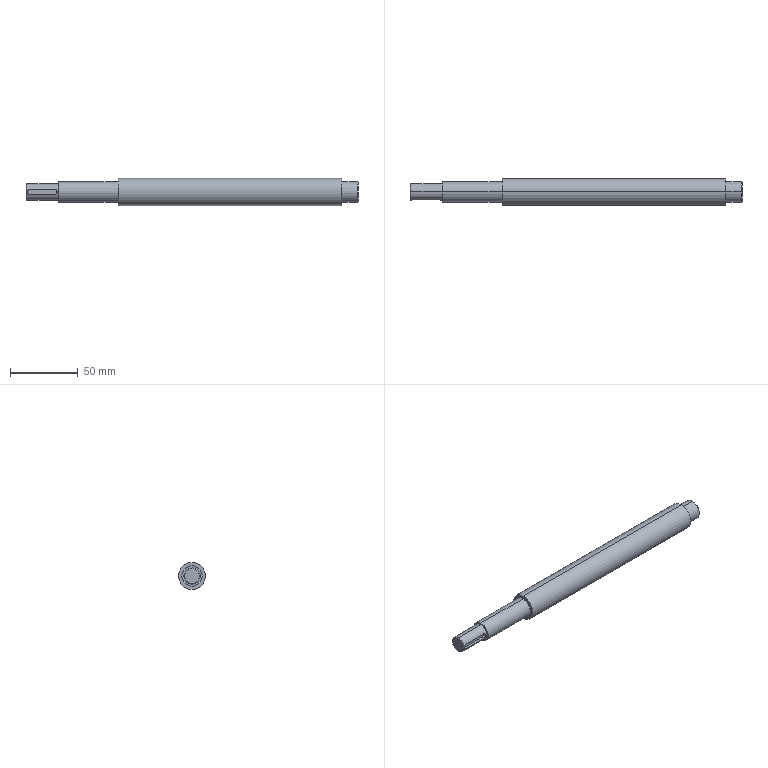Part | SolidWorks | features Chamfer 1, ICE 1, Revolution 1 | 1 solid | 22 faces | box 245 x 20 x 20 mm | volume 64259 mm3 | cylinder 10 | plane 8 | cone 4 | commonest cylinder face diameters 15 x4 4 x2 12 x2 20 x2
STEP:
#1=CARTESIAN_POINT('',(0.,0.,5.5));
#2=VERTEX_POINT('',#1);
#3=CARTESIAN_POINT('',(0.,0.,-5.5));
#4=VERTEX_POINT('',#3);
#5=CARTESIAN_POINT('',(0.,0.,0.));
#6=DIRECTION('',(-1.,0.,0.));
#7=DIRECTION('',(0.,0.,-1.));
#8=AXIS2_PLACEMENT_3D('',#5,#6,#7);
#9=CIRCLE('',#8,5.5);
#10=EDGE_CURVE('',#2,#4,#9,.T.);
#11=ORIENTED_EDGE('',*,*,#10,.F.);
#12=CARTESIAN_POINT('',(0.5,0.,6.));
#13=VERTEX_POINT('',#12);
#14=CARTESIAN_POINT('',(0.,0.,5.5));
#15=DIRECTION('',(0.7071,0.,0.7071));
#16=VECTOR('',#15,1000.);
#17=LINE('',#14,#16);
#18=EDGE_CURVE('',#2,#13,#17,.T.);
#19=ORIENTED_EDGE('',*,*,#18,.T.);
#20=CARTESIAN_POINT('',(0.5,0.,-6.));
#21=VERTEX_POINT('',#20);
#22=CARTESIAN_POINT('',(0.5,0.,0.));
#23=DIRECTION('',(1.,0.,0.));
#24=DIRECTION('',(0.,0.,-1.));
#25=AXIS2_PLACEMENT_3D('',#22,#23,#24);
#26=CIRCLE('',#25,6.);
#27=EDGE_CURVE('',#21,#13,#26,.T.);
#28=ORIENTED_EDGE('',*,*,#27,.F.);
#29=CARTESIAN_POINT('',(0.,0.,-5.5));
#30=DIRECTION('',(0.7071,0.,-0.7071));
#31=VECTOR('',#30,1000.);
#32=LINE('',#29,#31);
#33=EDGE_CURVE('',#4,#21,#32,.T.);
#34=ORIENTED_EDGE('',*,*,#33,.F.);
#35=EDGE_LOOP('',(#11,#19,#28,#34));
#36=FACE_OUTER_BOUND('',#35,.T.);
#37=CARTESIAN_POINT('',(0.,0.,0.));
#38=DIRECTION('',(1.,0.,0.));
#39=DIRECTION('',(0.,0.,-1.));
#40=AXIS2_PLACEMENT_3D('',#37,#38,#39);
#41=CONICAL_SURFACE('',#40,5.5,0.7854);
#42=ADVANCED_FACE('',(#36),#41,.T.);
#43=CARTESIAN_POINT('',(245.,0.,-7.));
#44=VERTEX_POINT('',#43);
#45=CARTESIAN_POINT('',(245.,0.,7.));
#46=VERTEX_POINT('',#45);
#47=CARTESIAN_POINT('',(245.,0.,0.));
#48=DIRECTION('',(1.,0.,0.));
#49=DIRECTION('',(0.,0.,1.));
#50=AXIS2_PLACEMENT_3D('',#47,#48,#49);
#51=CIRCLE('',#50,7.);
#52=EDGE_CURVE('',#44,#46,#51,.T.);
#53=ORIENTED_EDGE('',*,*,#52,.F.);
#54=CARTESIAN_POINT('',(244.5,0.,-7.5));
#55=VERTEX_POINT('',#54);
#56=CARTESIAN_POINT('',(244.5,0.,-7.5));
#57=DIRECTION('',(-0.7071,0.,-0.7071));
#58=VECTOR('',#57,1000.);
#59=LINE('',#56,#58);
#60=EDGE_CURVE('',#44,#55,#59,.T.);
#61=ORIENTED_EDGE('',*,*,#60,.T.);
#62=CARTESIAN_POINT('',(244.5,0.,7.5));
#63=VERTEX_POINT('',#62);
#64=CARTESIAN_POINT('',(244.5,0.,0.));
#65=DIRECTION('',(-1.,0.,0.));
#66=DIRECTION('',(0.,0.,1.));
#67=AXIS2_PLACEMENT_3D('',#64,#65,#66);
#68=CIRCLE('',#67,7.5);
#69=EDGE_CURVE('',#63,#55,#68,.T.);
#70=ORIENTED_EDGE('',*,*,#69,.F.);
#71=CARTESIAN_POINT('',(244.5,0.,7.5));
#72=DIRECTION('',(-0.7071,0.,0.7071));
#73=VECTOR('',#72,1000.);
#74=LINE('',#71,#73);
#75=EDGE_CURVE('',#46,#63,#74,.T.);
#76=ORIENTED_EDGE('',*,*,#75,.F.);
#77=EDGE_LOOP('',(#53,#61,#70,#76));
#78=FACE_OUTER_BOUND('',#77,.T.);
#79=CARTESIAN_POINT('',(244.5,0.,0.));
#80=DIRECTION('',(-1.,0.,0.));
#81=DIRECTION('',(0.,0.,1.));
#82=AXIS2_PLACEMENT_3D('',#79,#80,#81);
#83=CONICAL_SURFACE('',#82,7.5,0.7854);
#84=ADVANCED_FACE('',(#78),#83,.T.);
#85=ORIENTED_EDGE('',*,*,#69,.T.);
#86=CARTESIAN_POINT('',(233.,0.,-7.5));
#87=VERTEX_POINT('',#86);
#88=CARTESIAN_POINT('',(0.,0.,-7.5));
#89=DIRECTION('',(-1.,0.,0.));
#90=VECTOR('',#89,1000.);
#91=LINE('',#88,#90);
#92=EDGE_CURVE('',#55,#87,#91,.T.);
#93=ORIENTED_EDGE('',*,*,#92,.T.);
#94=CARTESIAN_POINT('',(233.,0.,7.5));
#95=VERTEX_POINT('',#94);
#96=CARTESIAN_POINT('',(233.,0.,0.));
#97=DIRECTION('',(-1.,0.,0.));
#98=DIRECTION('',(0.,0.,1.));
#99=AXIS2_PLACEMENT_3D('',#96,#97,#98);
#100=CIRCLE('',#99,7.5);
#101=EDGE_CURVE('',#95,#87,#100,.T.);
#102=ORIENTED_EDGE('',*,*,#101,.F.);
#103=CARTESIAN_POINT('',(0.,0.,7.5));
#104=DIRECTION('',(-1.,0.,0.));
#105=VECTOR('',#104,1000.);
#106=LINE('',#103,#105);
#107=EDGE_CURVE('',#63,#95,#106,.T.);
#108=ORIENTED_EDGE('',*,*,#107,.F.);
#109=EDGE_LOOP('',(#85,#93,#102,#108));
#110=FACE_OUTER_BOUND('',#109,.T.);
#111=CARTESIAN_POINT('',(0.,0.,0.));
#112=DIRECTION('',(-1.,0.,0.));
#113=DIRECTION('',(0.,0.,1.));
#114=AXIS2_PLACEMENT_3D('',#111,#112,#113);
#115=CYLINDRICAL_SURFACE('',#114,7.5);
#116=ADVANCED_FACE('',(#110),#115,.T.);
#117=CARTESIAN_POINT('',(233.,0.,10.));
#118=VERTEX_POINT('',#117);
#119=CARTESIAN_POINT('',(233.,0.,-10.));
#120=VERTEX_POINT('',#119);
#121=CARTESIAN_POINT('',(233.,0.,0.));
#122=DIRECTION('',(-1.,0.,0.));
#123=DIRECTION('',(0.,0.,1.));
#124=AXIS2_PLACEMENT_3D('',#121,#122,#123);
#125=CIRCLE('',#124,10.);
#126=EDGE_CURVE('',#118,#120,#125,.T.);
#127=ORIENTED_EDGE('',*,*,#126,.T.);
#128=CARTESIAN_POINT('',(68.,0.,-10.));
#129=VERTEX_POINT('',#128);
#130=CARTESIAN_POINT('',(0.,0.,-10.));
#131=DIRECTION('',(-1.,0.,0.));
#132=VECTOR('',#131,1000.);
#133=LINE('',#130,#132);
#134=EDGE_CURVE('',#120,#129,#133,.T.);
#135=ORIENTED_EDGE('',*,*,#134,.T.);
#136=CARTESIAN_POINT('',(68.,0.,10.));
#137=VERTEX_POINT('',#136);
#138=CARTESIAN_POINT('',(68.,0.,0.));
#139=DIRECTION('',(-1.,0.,0.));
#140=DIRECTION('',(0.,0.,1.));
#141=AXIS2_PLACEMENT_3D('',#138,#139,#140);
#142=CIRCLE('',#141,10.);
#143=EDGE_CURVE('',#137,#129,#142,.T.);
#144=ORIENTED_EDGE('',*,*,#143,.F.);
#145=CARTESIAN_POINT('',(0.,0.,10.));
#146=DIRECTION('',(-1.,0.,0.));
#147=VECTOR('',#146,1000.);
#148=LINE('',#145,#147);
#149=EDGE_CURVE('',#118,#137,#148,.T.);
#150=ORIENTED_EDGE('',*,*,#149,.F.);
#151=EDGE_LOOP('',(#127,#135,#144,#150));
#152=FACE_OUTER_BOUND('',#151,.T.);
#153=CARTESIAN_POINT('',(0.,0.,0.));
#154=DIRECTION('',(-1.,0.,0.));
#155=DIRECTION('',(0.,0.,1.));
#156=AXIS2_PLACEMENT_3D('',#153,#154,#155);
#157=CYLINDRICAL_SURFACE('',#156,10.);
#158=ADVANCED_FACE('',(#152),#157,.T.);
#159=CARTESIAN_POINT('',(68.,0.,7.5));
#160=VERTEX_POINT('',#159);
#161=CARTESIAN_POINT('',(68.,0.,-7.5));
#162=VERTEX_POINT('',#161);
#163=CARTESIAN_POINT('',(68.,0.,0.));
#164=DIRECTION('',(-1.,0.,0.));
#165=DIRECTION('',(0.,0.,1.));
#166=AXIS2_PLACEMENT_3D('',#163,#164,#165);
#167=CIRCLE('',#166,7.5);
#168=EDGE_CURVE('',#160,#162,#167,.T.);
#169=ORIENTED_EDGE('',*,*,#168,.T.);
#170=CARTESIAN_POINT('',(24.,0.,-7.5));
#171=VERTEX_POINT('',#170);
#172=CARTESIAN_POINT('',(0.,0.,-7.5));
#173=DIRECTION('',(-1.,0.,0.));
#174=VECTOR('',#173,1000.);
#175=LINE('',#172,#174);
#176=EDGE_CURVE('',#162,#171,#175,.T.);
#177=ORIENTED_EDGE('',*,*,#176,.T.);
#178=CARTESIAN_POINT('',(24.,0.,7.5));
#179=VERTEX_POINT('',#178);
#180=CARTESIAN_POINT('',(24.,0.,0.));
#181=DIRECTION('',(-1.,0.,0.));
#182=DIRECTION('',(0.,0.,1.));
#183=AXIS2_PLACEMENT_3D('',#180,#181,#182);
#184=CIRCLE('',#183,7.5);
#185=EDGE_CURVE('',#179,#171,#184,.T.);
#186=ORIENTED_EDGE('',*,*,#185,.F.);
#187=CARTESIAN_POINT('',(0.,0.,7.5));
#188=DIRECTION('',(-1.,0.,0.));
#189=VECTOR('',#188,1000.);
#190=LINE('',#187,#189);
#191=EDGE_CURVE('',#160,#179,#190,.T.);
#192=ORIENTED_EDGE('',*,*,#191,.F.);
#193=EDGE_LOOP('',(#169,#177,#186,#192));
#194=FACE_OUTER_BOUND('',#193,.T.);
#195=CARTESIAN_POINT('',(0.,0.,0.));
#196=DIRECTION('',(-1.,0.,0.));
#197=DIRECTION('',(0.,0.,1.));
#198=AXIS2_PLACEMENT_3D('',#195,#196,#197);
#199=CYLINDRICAL_SURFACE('',#198,7.5);
#200=ADVANCED_FACE('',(#194),#199,.T.);
#201=CARTESIAN_POINT('',(24.,0.,6.));
#202=VERTEX_POINT('',#201);
#203=CARTESIAN_POINT('',(24.,0.,-6.));
#204=VERTEX_POINT('',#203);
#205=CARTESIAN_POINT('',(24.,0.,0.));
#206=DIRECTION('',(-1.,0.,0.));
#207=DIRECTION('',(0.,0.,1.));
#208=AXIS2_PLACEMENT_3D('',#205,#206,#207);
#209=CIRCLE('',#208,6.);
#210=EDGE_CURVE('',#202,#204,#209,.T.);
#211=ORIENTED_EDGE('',*,*,#210,.T.);
#212=CARTESIAN_POINT('',(0.,0.,-6.));
#213=DIRECTION('',(-1.,0.,0.));
#214=VECTOR('',#213,1000.);
#215=LINE('',#212,#214);
#216=EDGE_CURVE('',#204,#21,#215,.T.);
#217=ORIENTED_EDGE('',*,*,#216,.T.);
#218=ORIENTED_EDGE('',*,*,#27,.T.);
#219=CARTESIAN_POINT('',(0.,0.,6.));
#220=DIRECTION('',(-1.,0.,0.));
#221=VECTOR('',#220,1000.);
#222=LINE('',#219,#221);
#223=EDGE_CURVE('',#202,#13,#222,.T.);
#224=ORIENTED_EDGE('',*,*,#223,.F.);
#225=EDGE_LOOP('',(#211,#217,#218,#224));
#226=FACE_OUTER_BOUND('',#225,.T.);
#227=CARTESIAN_POINT('',(0.,0.,0.));
#228=DIRECTION('',(-1.,0.,0.));
#229=DIRECTION('',(0.,0.,1.));
#230=AXIS2_PLACEMENT_3D('',#227,#228,#229);
#231=CYLINDRICAL_SURFACE('',#230,6.);
#232=ADVANCED_FACE('',(#226),#231,.T.);
#233=CARTESIAN_POINT('',(0.,0.,0.));
#234=DIRECTION('',(-1.,0.,0.));
#235=DIRECTION('',(0.,0.,-1.));
#236=AXIS2_PLACEMENT_3D('',#233,#234,#235);
#237=CIRCLE('',#236,5.5);
#238=EDGE_CURVE('',#4,#2,#237,.T.);
#239=ORIENTED_EDGE('',*,*,#238,.T.);
#240=ORIENTED_EDGE('',*,*,#10,.T.);
#241=EDGE_LOOP('',(#239,#240));
#242=FACE_OUTER_BOUND('',#241,.T.);
#243=CARTESIAN_POINT('',(0.,0.,0.));
#244=DIRECTION('',(1.,0.,0.));
#245=DIRECTION('',(0.,0.,-1.));
#246=AXIS2_PLACEMENT_3D('',#243,#244,#245);
#247=PLANE('',#246);
#248=ADVANCED_FACE('',(#242),#247,.F.);
#249=ORIENTED_EDGE('',*,*,#216,.F.);
#250=CARTESIAN_POINT('',(24.,0.,0.));
#251=DIRECTION('',(-1.,0.,0.));
#252=DIRECTION('',(0.,0.,1.));
#253=AXIS2_PLACEMENT_3D('',#250,#251,#252);
#254=CIRCLE('',#253,6.);
#255=EDGE_CURVE('',#204,#202,#254,.T.);
#256=ORIENTED_EDGE('',*,*,#255,.T.);
#257=ORIENTED_EDGE('',*,*,#223,.T.);
#258=CARTESIAN_POINT('',(0.5,0.,0.));
#259=DIRECTION('',(1.,0.,0.));
#260=DIRECTION('',(0.,0.,-1.));
#261=AXIS2_PLACEMENT_3D('',#258,#259,#260);
#262=CIRCLE('',#261,6.);
#263=EDGE_CURVE('',#13,#21,#262,.T.);
#264=ORIENTED_EDGE('',*,*,#263,.T.);
#265=EDGE_LOOP('',(#249,#256,#257,#264));
#266=FACE_OUTER_BOUND('',#265,.T.);
#267=CARTESIAN_POINT('',(21.,-5.657,-2.));
#268=VERTEX_POINT('',#267);
#269=CARTESIAN_POINT('',(3.,-5.657,-2.));
#270=VERTEX_POINT('',#269);
#271=CARTESIAN_POINT('',(0.,-5.657,-2.));
#272=DIRECTION('',(-1.,0.,0.));
#273=VECTOR('',#272,1000.);
#274=LINE('',#271,#273);
#275=EDGE_CURVE('',#268,#270,#274,.T.);
#276=ORIENTED_EDGE('',*,*,#275,.T.);
#277=CARTESIAN_POINT('',(3.,-5.657,2.));
#278=VERTEX_POINT('',#277);
#279=CARTESIAN_POINT('',(3.,-5.657,-2.));
#280=CARTESIAN_POINT('',(2.867,-5.657,-2.));
#281=CARTESIAN_POINT('',(2.736,-5.662,-1.987));
#282=CARTESIAN_POINT('',(2.479,-5.679,-1.935));
#283=CARTESIAN_POINT('',(2.352,-5.693,-1.897));
#284=CARTESIAN_POINT('',(2.11,-5.725,-1.796));
#285=CARTESIAN_POINT('',(1.996,-5.744,-1.735));
#286=CARTESIAN_POINT('',(1.779,-5.786,-1.59));
#287=CARTESIAN_POINT('',(1.677,-5.809,-1.506));
#288=CARTESIAN_POINT('',(1.403,-5.875,-1.231));
#289=CARTESIAN_POINT('',(1.254,-5.919,-1.01));
#290=CARTESIAN_POINT('',(1.104,-5.966,-0.6496));
#291=CARTESIAN_POINT('',(1.065,-5.979,-0.5226));
#292=CARTESIAN_POINT('',(1.013,-5.996,-0.264));
#293=CARTESIAN_POINT('',(1.,-6.,-0.1336));
#294=CARTESIAN_POINT('',(0.9999,-6.,0.1294));
#295=CARTESIAN_POINT('',(1.013,-5.996,0.2629));
#296=CARTESIAN_POINT('',(1.064,-5.979,0.5202));
#297=CARTESIAN_POINT('',(1.102,-5.966,0.6454));
#298=CARTESIAN_POINT('',(1.204,-5.935,0.8889));
#299=CARTESIAN_POINT('',(1.266,-5.916,1.004));
#300=CARTESIAN_POINT('',(1.41,-5.876,1.22));
#301=CARTESIAN_POINT('',(1.493,-5.853,1.322));
#302=CARTESIAN_POINT('',(1.677,-5.809,1.506));
#303=CARTESIAN_POINT('',(1.777,-5.787,1.588));
#304=CARTESIAN_POINT('',(1.993,-5.745,1.733));
#305=CARTESIAN_POINT('',(2.11,-5.725,1.796));
#306=CARTESIAN_POINT('',(2.471,-5.677,1.946));
#307=CARTESIAN_POINT('',(2.734,-5.657,2.));
#308=CARTESIAN_POINT('',(3.,-5.657,2.));
#309=B_SPLINE_CURVE_WITH_KNOTS('',3,(#279,#280,#281,#282,#283,#284,#285,#286,#287,#288,#289,#290,#291,#292,#293,#294,#295,#296,#297,#298,#299,#300,#301,#302,#303,#304,#305,#306,#307,#308),.UNSPECIFIED.,.F.,.F.,(4,2,2,2,2,2,2,2,2,2,2,2,2,2,4),(0.,0.0003935,0.000787,0.00118,0.001574,0.002361,0.002754,0.003148,0.003541,0.003935,0.004328,0.004722,0.005115,0.005509,0.006296),.UNSPECIFIED.);
#310=EDGE_CURVE('',#270,#278,#309,.T.);
#311=ORIENTED_EDGE('',*,*,#310,.T.);
#312=CARTESIAN_POINT('',(21.,-5.657,2.));
#313=VERTEX_POINT('',#312);
#314=CARTESIAN_POINT('',(0.,-5.657,2.));
#315=DIRECTION('',(1.,0.,0.));
#316=VECTOR('',#315,1000.);
#317=LINE('',#314,#316);
#318=EDGE_CURVE('',#278,#313,#317,.T.);
#319=ORIENTED_EDGE('',*,*,#318,.T.);
#320=CARTESIAN_POINT('',(21.,-5.657,2.));
#321=CARTESIAN_POINT('',(21.133,-5.657,2.));
#322=CARTESIAN_POINT('',(21.264,-5.662,1.987));
#323=CARTESIAN_POINT('',(21.521,-5.679,1.935));
#324=CARTESIAN_POINT('',(21.648,-5.693,1.897));
#325=CARTESIAN_POINT('',(21.89,-5.725,1.796));
#326=CARTESIAN_POINT('',(22.004,-5.744,1.735));
#327=CARTESIAN_POINT('',(22.221,-5.786,1.59));
#328=CARTESIAN_POINT('',(22.323,-5.809,1.506));
#329=CARTESIAN_POINT('',(22.597,-5.875,1.231));
#330=CARTESIAN_POINT('',(22.746,-5.919,1.01));
#331=CARTESIAN_POINT('',(22.896,-5.966,0.6496));
#332=CARTESIAN_POINT('',(22.935,-5.979,0.5226));
#333=CARTESIAN_POINT('',(22.987,-5.996,0.264));
#334=CARTESIAN_POINT('',(23.,-6.,0.1336));
#335=CARTESIAN_POINT('',(23.,-6.,-0.1294));
#336=CARTESIAN_POINT('',(22.987,-5.996,-0.2629));
#337=CARTESIAN_POINT('',(22.936,-5.979,-0.5202));
#338=CARTESIAN_POINT('',(22.898,-5.966,-0.6454));
#339=CARTESIAN_POINT('',(22.796,-5.935,-0.8889));
#340=CARTESIAN_POINT('',(22.734,-5.916,-1.004));
#341=CARTESIAN_POINT('',(22.59,-5.876,-1.22));
#342=CARTESIAN_POINT('',(22.507,-5.853,-1.322));
#343=CARTESIAN_POINT('',(22.323,-5.809,-1.506));
#344=CARTESIAN_POINT('',(22.223,-5.787,-1.588));
#345=CARTESIAN_POINT('',(22.007,-5.745,-1.733));
#346=CARTESIAN_POINT('',(21.89,-5.725,-1.796));
#347=CARTESIAN_POINT('',(21.529,-5.677,-1.946));
#348=CARTESIAN_POINT('',(21.266,-5.657,-2.));
#349=CARTESIAN_POINT('',(21.,-5.657,-2.));
#350=B_SPLINE_CURVE_WITH_KNOTS('',3,(#320,#321,#322,#323,#324,#325,#326,#327,#328,#329,#330,#331,#332,#333,#334,#335,#336,#337,#338,#339,#340,#341,#342,#343,#344,#345,#346,#347,#348,#349),.UNSPECIFIED.,.F.,.F.,(4,2,2,2,2,2,2,2,2,2,2,2,2,2,4),(0.,0.0003935,0.000787,0.00118,0.001574,0.002361,0.002754,0.003148,0.003541,0.003935,0.004328,0.004722,0.005115,0.005509,0.006296),.UNSPECIFIED.);
#351=EDGE_CURVE('',#313,#268,#350,.T.);
#352=ORIENTED_EDGE('',*,*,#351,.T.);
#353=EDGE_LOOP('',(#276,#311,#319,#352));
#354=FACE_BOUND('',#353,.T.);
#355=CARTESIAN_POINT('',(0.,0.,0.));
#356=DIRECTION('',(-1.,0.,0.));
#357=DIRECTION('',(0.,0.,1.));
#358=AXIS2_PLACEMENT_3D('',#355,#356,#357);
#359=CYLINDRICAL_SURFACE('',#358,6.);
#360=ADVANCED_FACE('',(#266,#354),#359,.T.);
#361=ORIENTED_EDGE('',*,*,#210,.F.);
#362=ORIENTED_EDGE('',*,*,#255,.F.);
#363=EDGE_LOOP('',(#361,#362));
#364=FACE_BOUND('',#363,.T.);
#365=ORIENTED_EDGE('',*,*,#185,.T.);
#366=CARTESIAN_POINT('',(24.,0.,0.));
#367=DIRECTION('',(-1.,0.,0.));
#368=DIRECTION('',(0.,0.,1.));
#369=AXIS2_PLACEMENT_3D('',#366,#367,#368);
#370=CIRCLE('',#369,7.5);
#371=EDGE_CURVE('',#171,#179,#370,.T.);
#372=ORIENTED_EDGE('',*,*,#371,.T.);
#373=EDGE_LOOP('',(#365,#372));
#374=FACE_OUTER_BOUND('',#373,.T.);
#375=CARTESIAN_POINT('',(24.,0.,-6.));
#376=DIRECTION('',(1.,0.,0.));
#377=DIRECTION('',(0.,0.,-1.));
#378=AXIS2_PLACEMENT_3D('',#375,#376,#377);
#379=PLANE('',#378);
#380=ADVANCED_FACE('',(#364,#374),#379,.F.);
#381=ORIENTED_EDGE('',*,*,#176,.F.);
#382=CARTESIAN_POINT('',(68.,0.,0.));
#383=DIRECTION('',(-1.,0.,0.));
#384=DIRECTION('',(0.,0.,1.));
#385=AXIS2_PLACEMENT_3D('',#382,#383,#384);
#386=CIRCLE('',#385,7.5);
#387=EDGE_CURVE('',#162,#160,#386,.T.);
#388=ORIENTED_EDGE('',*,*,#387,.T.);
#389=ORIENTED_EDGE('',*,*,#191,.T.);
#390=ORIENTED_EDGE('',*,*,#371,.F.);
#391=EDGE_LOOP('',(#381,#388,#389,#390));
#392=FACE_OUTER_BOUND('',#391,.T.);
#393=CARTESIAN_POINT('',(0.,0.,0.));
#394=DIRECTION('',(-1.,0.,0.));
#395=DIRECTION('',(0.,0.,1.));
#396=AXIS2_PLACEMENT_3D('',#393,#394,#395);
#397=CYLINDRICAL_SURFACE('',#396,7.5);
#398=ADVANCED_FACE('',(#392),#397,.T.);
#399=ORIENTED_EDGE('',*,*,#168,.F.);
#400=ORIENTED_EDGE('',*,*,#387,.F.);
#401=EDGE_LOOP('',(#399,#400));
#402=FACE_BOUND('',#401,.T.);
#403=ORIENTED_EDGE('',*,*,#143,.T.);
#404=CARTESIAN_POINT('',(68.,0.,0.));
#405=DIRECTION('',(-1.,0.,0.));
#406=DIRECTION('',(0.,0.,1.));
#407=AXIS2_PLACEMENT_3D('',#404,#405,#406);
#408=CIRCLE('',#407,10.);
#409=EDGE_CURVE('',#129,#137,#408,.T.);
#410=ORIENTED_EDGE('',*,*,#409,.T.);
#411=EDGE_LOOP('',(#403,#410));
#412=FACE_OUTER_BOUND('',#411,.T.);
#413=CARTESIAN_POINT('',(68.,0.,-7.5));
#414=DIRECTION('',(1.,0.,0.));
#415=DIRECTION('',(0.,0.,-1.));
#416=AXIS2_PLACEMENT_3D('',#413,#414,#415);
#417=PLANE('',#416);
#418=ADVANCED_FACE('',(#402,#412),#417,.F.);
#419=ORIENTED_EDGE('',*,*,#134,.F.);
#420=CARTESIAN_POINT('',(233.,0.,0.));
#421=DIRECTION('',(-1.,0.,0.));
#422=DIRECTION('',(0.,0.,1.));
#423=AXIS2_PLACEMENT_3D('',#420,#421,#422);
#424=CIRCLE('',#423,10.);
#425=EDGE_CURVE('',#120,#118,#424,.T.);
#426=ORIENTED_EDGE('',*,*,#425,.T.);
#427=ORIENTED_EDGE('',*,*,#149,.T.);
#428=ORIENTED_EDGE('',*,*,#409,.F.);
#429=EDGE_LOOP('',(#419,#426,#427,#428));
#430=FACE_OUTER_BOUND('',#429,.T.);
#431=CARTESIAN_POINT('',(0.,0.,0.));
#432=DIRECTION('',(-1.,0.,0.));
#433=DIRECTION('',(0.,0.,1.));
#434=AXIS2_PLACEMENT_3D('',#431,#432,#433);
#435=CYLINDRICAL_SURFACE('',#434,10.);
#436=ADVANCED_FACE('',(#430),#435,.T.);
#437=ORIENTED_EDGE('',*,*,#126,.F.);
#438=ORIENTED_EDGE('',*,*,#425,.F.);
#439=EDGE_LOOP('',(#437,#438));
#440=FACE_OUTER_BOUND('',#439,.T.);
#441=ORIENTED_EDGE('',*,*,#101,.T.);
#442=CARTESIAN_POINT('',(233.,0.,0.));
#443=DIRECTION('',(-1.,0.,0.));
#444=DIRECTION('',(0.,0.,1.));
#445=AXIS2_PLACEMENT_3D('',#442,#443,#444);
#446=CIRCLE('',#445,7.5);
#447=EDGE_CURVE('',#87,#95,#446,.T.);
#448=ORIENTED_EDGE('',*,*,#447,.T.);
#449=EDGE_LOOP('',(#441,#448));
#450=FACE_BOUND('',#449,.T.);
#451=CARTESIAN_POINT('',(233.,0.,-10.));
#452=DIRECTION('',(-1.,0.,0.));
#453=DIRECTION('',(0.,0.,1.));
#454=AXIS2_PLACEMENT_3D('',#451,#452,#453);
#455=PLANE('',#454);
#456=ADVANCED_FACE('',(#440,#450),#455,.F.);
#457=ORIENTED_EDGE('',*,*,#92,.F.);
#458=CARTESIAN_POINT('',(244.5,0.,0.));
#459=DIRECTION('',(-1.,0.,0.));
#460=DIRECTION('',(0.,0.,1.));
#461=AXIS2_PLACEMENT_3D('',#458,#459,#460);
#462=CIRCLE('',#461,7.5);
#463=EDGE_CURVE('',#55,#63,#462,.T.);
#464=ORIENTED_EDGE('',*,*,#463,.T.);
#465=ORIENTED_EDGE('',*,*,#107,.T.);
#466=ORIENTED_EDGE('',*,*,#447,.F.);
#467=EDGE_LOOP('',(#457,#464,#465,#466));
#468=FACE_OUTER_BOUND('',#467,.T.);
#469=CARTESIAN_POINT('',(0.,0.,0.));
#470=DIRECTION('',(-1.,0.,0.));
#471=DIRECTION('',(0.,0.,1.));
#472=AXIS2_PLACEMENT_3D('',#469,#470,#471);
#473=CYLINDRICAL_SURFACE('',#472,7.5);
#474=ADVANCED_FACE('',(#468),#473,.T.);
#475=CARTESIAN_POINT('',(245.,0.,0.));
#476=DIRECTION('',(1.,0.,0.));
#477=DIRECTION('',(0.,0.,1.));
#478=AXIS2_PLACEMENT_3D('',#475,#476,#477);
#479=CIRCLE('',#478,7.);
#480=EDGE_CURVE('',#46,#44,#479,.T.);
#481=ORIENTED_EDGE('',*,*,#480,.T.);
#482=ORIENTED_EDGE('',*,*,#52,.T.);
#483=EDGE_LOOP('',(#481,#482));
#484=FACE_OUTER_BOUND('',#483,.T.);
#485=CARTESIAN_POINT('',(245.,0.,-7.5));
#486=DIRECTION('',(-1.,0.,0.));
#487=DIRECTION('',(0.,0.,1.));
#488=AXIS2_PLACEMENT_3D('',#485,#486,#487);
#489=PLANE('',#488);
#490=ADVANCED_FACE('',(#484),#489,.F.);
#491=CARTESIAN_POINT('',(21.,-3.8,2.));
#492=VERTEX_POINT('',#491);
#493=CARTESIAN_POINT('',(21.,-3.8,2.));
#494=DIRECTION('',(0.,-1.,0.));
#495=VECTOR('',#494,1000.);
#496=LINE('',#493,#495);
#497=EDGE_CURVE('',#492,#313,#496,.T.);
#498=ORIENTED_EDGE('',*,*,#497,.F.);
#499=CARTESIAN_POINT('',(21.,-3.8,-2.));
#500=VERTEX_POINT('',#499);
#501=CARTESIAN_POINT('',(21.,-3.8,0.));
#502=DIRECTION('',(0.,-1.,0.));
#503=DIRECTION('',(0.,0.,-1.));
#504=AXIS2_PLACEMENT_3D('',#501,#502,#503);
#505=CIRCLE('',#504,2.);
#506=EDGE_CURVE('',#500,#492,#505,.T.);
#507=ORIENTED_EDGE('',*,*,#506,.F.);
#508=CARTESIAN_POINT('',(21.,-3.8,-2.));
#509=DIRECTION('',(0.,-1.,0.));
#510=VECTOR('',#509,1000.);
#511=LINE('',#508,#510);
#512=EDGE_CURVE('',#500,#268,#511,.T.);
#513=ORIENTED_EDGE('',*,*,#512,.T.);
#514=ORIENTED_EDGE('',*,*,#351,.F.);
#515=EDGE_LOOP('',(#498,#507,#513,#514));
#516=FACE_OUTER_BOUND('',#515,.T.);
#517=CARTESIAN_POINT('',(21.,-3.8,0.));
#518=DIRECTION('',(0.,-1.,0.));
#519=DIRECTION('',(0.,0.,-1.));
#520=AXIS2_PLACEMENT_3D('',#517,#518,#519);
#521=CYLINDRICAL_SURFACE('',#520,2.);
#522=ADVANCED_FACE('',(#516),#521,.F.);
#523=ORIENTED_EDGE('',*,*,#512,.F.);
#524=CARTESIAN_POINT('',(3.,-3.8,-2.));
#525=VERTEX_POINT('',#524);
#526=CARTESIAN_POINT('',(21.,-3.8,-2.));
#527=DIRECTION('',(1.,0.,0.));
#528=VECTOR('',#527,1000.);
#529=LINE('',#526,#528);
#530=EDGE_CURVE('',#525,#500,#529,.T.);
#531=ORIENTED_EDGE('',*,*,#530,.F.);
#532=CARTESIAN_POINT('',(3.,-3.8,-2.));
#533=DIRECTION('',(0.,-1.,0.));
#534=VECTOR('',#533,1000.);
#535=LINE('',#532,#534);
#536=EDGE_CURVE('',#525,#270,#535,.T.);
#537=ORIENTED_EDGE('',*,*,#536,.T.);
#538=ORIENTED_EDGE('',*,*,#275,.F.);
#539=EDGE_LOOP('',(#523,#531,#537,#538));
#540=FACE_OUTER_BOUND('',#539,.T.);
#541=CARTESIAN_POINT('',(21.,-3.8,-2.));
#542=DIRECTION('',(0.,0.,-1.));
#543=DIRECTION('',(-1.,0.,0.));
#544=AXIS2_PLACEMENT_3D('',#541,#542,#543);
#545=PLANE('',#544);
#546=ADVANCED_FACE('',(#540),#545,.F.);
#547=ORIENTED_EDGE('',*,*,#536,.F.);
#548=CARTESIAN_POINT('',(3.,-3.8,2.));
#549=VERTEX_POINT('',#548);
#550=CARTESIAN_POINT('',(3.,-3.8,0.));
#551=DIRECTION('',(0.,-1.,0.));
#552=DIRECTION('',(0.,0.,-1.));
#553=AXIS2_PLACEMENT_3D('',#550,#551,#552);
#554=CIRCLE('',#553,2.);
#555=EDGE_CURVE('',#549,#525,#554,.T.);
#556=ORIENTED_EDGE('',*,*,#555,.F.);
#557=CARTESIAN_POINT('',(3.,-3.8,2.));
#558=DIRECTION('',(0.,-1.,0.));
#559=VECTOR('',#558,1000.);
#560=LINE('',#557,#559);
#561=EDGE_CURVE('',#549,#278,#560,.T.);
#562=ORIENTED_EDGE('',*,*,#561,.T.);
#563=ORIENTED_EDGE('',*,*,#310,.F.);
#564=EDGE_LOOP('',(#547,#556,#562,#563));
#565=FACE_OUTER_BOUND('',#564,.T.);
#566=CARTESIAN_POINT('',(3.,-3.8,0.));
#567=DIRECTION('',(0.,-1.,0.));
#568=DIRECTION('',(0.,0.,-1.));
#569=AXIS2_PLACEMENT_3D('',#566,#567,#568);
#570=CYLINDRICAL_SURFACE('',#569,2.);
#571=ADVANCED_FACE('',(#565),#570,.F.);
#572=ORIENTED_EDGE('',*,*,#561,.F.);
#573=CARTESIAN_POINT('',(21.,-3.8,2.));
#574=DIRECTION('',(-1.,0.,0.));
#575=VECTOR('',#574,1000.);
#576=LINE('',#573,#575);
#577=EDGE_CURVE('',#492,#549,#576,.T.);
#578=ORIENTED_EDGE('',*,*,#577,.F.);
#579=ORIENTED_EDGE('',*,*,#497,.T.);
#580=ORIENTED_EDGE('',*,*,#318,.F.);
#581=EDGE_LOOP('',(#572,#578,#579,#580));
#582=FACE_OUTER_BOUND('',#581,.T.);
#583=CARTESIAN_POINT('',(21.,-3.8,2.));
#584=DIRECTION('',(0.,0.,1.));
#585=DIRECTION('',(1.,0.,0.));
#586=AXIS2_PLACEMENT_3D('',#583,#584,#585);
#587=PLANE('',#586);
#588=ADVANCED_FACE('',(#582),#587,.F.);
#589=ORIENTED_EDGE('',*,*,#506,.T.);
#590=ORIENTED_EDGE('',*,*,#577,.T.);
#591=ORIENTED_EDGE('',*,*,#555,.T.);
#592=ORIENTED_EDGE('',*,*,#530,.T.);
#593=EDGE_LOOP('',(#589,#590,#591,#592));
#594=FACE_OUTER_BOUND('',#593,.T.);
#595=CARTESIAN_POINT('',(21.,-3.8,0.));
#596=DIRECTION('',(0.,-1.,0.));
#597=DIRECTION('',(0.,0.,-1.));
#598=AXIS2_PLACEMENT_3D('',#595,#596,#597);
#599=PLANE('',#598);
#600=ADVANCED_FACE('',(#594),#599,.T.);
#601=ORIENTED_EDGE('',*,*,#60,.F.);
#602=ORIENTED_EDGE('',*,*,#480,.F.);
#603=ORIENTED_EDGE('',*,*,#75,.T.);
#604=ORIENTED_EDGE('',*,*,#463,.F.);
#605=EDGE_LOOP('',(#601,#602,#603,#604));
#606=FACE_OUTER_BOUND('',#605,.T.);
#607=CARTESIAN_POINT('',(244.5,0.,0.));
#608=DIRECTION('',(-1.,0.,0.));
#609=DIRECTION('',(0.,0.,1.));
#610=AXIS2_PLACEMENT_3D('',#607,#608,#609);
#611=CONICAL_SURFACE('',#610,7.5,0.7854);
#612=ADVANCED_FACE('',(#606),#611,.T.);
#613=ORIENTED_EDGE('',*,*,#18,.F.);
#614=ORIENTED_EDGE('',*,*,#238,.F.);
#615=ORIENTED_EDGE('',*,*,#33,.T.);
#616=ORIENTED_EDGE('',*,*,#263,.F.);
#617=EDGE_LOOP('',(#613,#614,#615,#616));
#618=FACE_OUTER_BOUND('',#617,.T.);
#619=CARTESIAN_POINT('',(0.,0.,0.));
#620=DIRECTION('',(1.,0.,0.));
#621=DIRECTION('',(0.,0.,-1.));
#622=AXIS2_PLACEMENT_3D('',#619,#620,#621);
#623=CONICAL_SURFACE('',#622,5.5,0.7854);
#624=ADVANCED_FACE('',(#618),#623,.T.);
#625=CLOSED_SHELL('',(#42,#84,#116,#158,#200,#232,#248,#360,#380,#398,#418,#436,#456,#474,#490,#522,#546,#571,#588,#600,#612,#624));
#626=MANIFOLD_SOLID_BREP('',#625);
#627=CARTESIAN_POINT('',(0.,0.,0.));
#628=DIRECTION('',(0.,0.,1.));
#629=DIRECTION('',(1.,0.,0.));
#630=AXIS2_PLACEMENT_3D('',#627,#628,#629);
#631=(LENGTH_UNIT()NAMED_UNIT(*)SI_UNIT(.MILLI.,.METRE.));
#632=UNCERTAINTY_MEASURE_WITH_UNIT(LENGTH_MEASURE(0.00001),#631,'','');
#633=(NAMED_UNIT(*)PLANE_ANGLE_UNIT()SI_UNIT($,.RADIAN.));
#634=(NAMED_UNIT(*)SI_UNIT($,.STERADIAN.)SOLID_ANGLE_UNIT());
#635=(GEOMETRIC_REPRESENTATION_CONTEXT(3)GLOBAL_UNCERTAINTY_ASSIGNED_CONTEXT((#632))GLOBAL_UNIT_ASSIGNED_CONTEXT((#631,#633,#634))REPRESENTATION_CONTEXT('',''));
#636=ADVANCED_BREP_SHAPE_REPRESENTATION('',(#626,#630),#635);